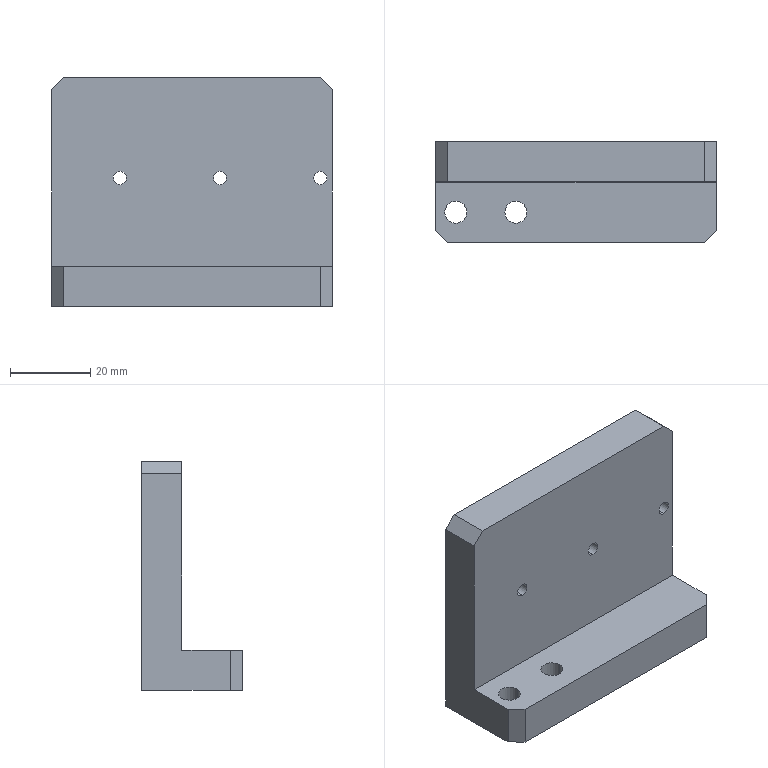Part | SolidWorks | features HoleWzd 2, Chamfer 1, Extrusion 1, ICE 1 | 1 solid | 22 faces | box 70 x 25 x 57 mm | volume 49488 mm3 | plane 12 | cylinder 10 | commonest cylinder face diameters 3.3 x6 5.5 x4
STEP:
#1=CARTESIAN_POINT('',(-17.75,-7.5,-28.5));
#2=VERTEX_POINT('',#1);
#3=CARTESIAN_POINT('',(-12.25,-7.5,-28.5));
#4=VERTEX_POINT('',#3);
#5=CARTESIAN_POINT('',(-15.,-7.5,-28.5));
#6=DIRECTION('',(0.,0.,1.));
#7=DIRECTION('',(1.,0.,0.));
#8=AXIS2_PLACEMENT_3D('',#5,#6,#7);
#9=CIRCLE('',#8,2.75);
#10=EDGE_CURVE('',#2,#4,#9,.T.);
#11=ORIENTED_EDGE('',*,*,#10,.F.);
#12=CARTESIAN_POINT('',(-17.75,-7.5,-18.5));
#13=VERTEX_POINT('',#12);
#14=CARTESIAN_POINT('',(-17.75,-7.5,-18.5));
#15=DIRECTION('',(0.,0.,1.));
#16=VECTOR('',#15,1000.);
#17=LINE('',#14,#16);
#18=EDGE_CURVE('',#2,#13,#17,.T.);
#19=ORIENTED_EDGE('',*,*,#18,.T.);
#20=CARTESIAN_POINT('',(-12.25,-7.5,-18.5));
#21=VERTEX_POINT('',#20);
#22=CARTESIAN_POINT('',(-15.,-7.5,-18.5));
#23=DIRECTION('',(0.,0.,1.));
#24=DIRECTION('',(1.,0.,0.));
#25=AXIS2_PLACEMENT_3D('',#22,#23,#24);
#26=CIRCLE('',#25,2.75);
#27=EDGE_CURVE('',#13,#21,#26,.T.);
#28=ORIENTED_EDGE('',*,*,#27,.T.);
#29=CARTESIAN_POINT('',(-12.25,-7.5,-18.5));
#30=DIRECTION('',(0.,0.,1.));
#31=VECTOR('',#30,1000.);
#32=LINE('',#29,#31);
#33=EDGE_CURVE('',#4,#21,#32,.T.);
#34=ORIENTED_EDGE('',*,*,#33,.F.);
#35=EDGE_LOOP('',(#11,#19,#28,#34));
#36=FACE_OUTER_BOUND('',#35,.T.);
#37=CARTESIAN_POINT('',(-15.,-7.5,-18.5));
#38=DIRECTION('',(0.,0.,1.));
#39=DIRECTION('',(1.,0.,0.));
#40=AXIS2_PLACEMENT_3D('',#37,#38,#39);
#41=CYLINDRICAL_SURFACE('',#40,2.75);
#42=ADVANCED_FACE('',(#36),#41,.F.);
#43=CARTESIAN_POINT('',(-32.75,-7.5,-28.5));
#44=VERTEX_POINT('',#43);
#45=CARTESIAN_POINT('',(-27.25,-7.5,-28.5));
#46=VERTEX_POINT('',#45);
#47=CARTESIAN_POINT('',(-30.,-7.5,-28.5));
#48=DIRECTION('',(0.,0.,1.));
#49=DIRECTION('',(1.,0.,0.));
#50=AXIS2_PLACEMENT_3D('',#47,#48,#49);
#51=CIRCLE('',#50,2.75);
#52=EDGE_CURVE('',#44,#46,#51,.T.);
#53=ORIENTED_EDGE('',*,*,#52,.F.);
#54=CARTESIAN_POINT('',(-32.75,-7.5,-18.5));
#55=VERTEX_POINT('',#54);
#56=CARTESIAN_POINT('',(-32.75,-7.5,-18.5));
#57=DIRECTION('',(0.,0.,1.));
#58=VECTOR('',#57,1000.);
#59=LINE('',#56,#58);
#60=EDGE_CURVE('',#44,#55,#59,.T.);
#61=ORIENTED_EDGE('',*,*,#60,.T.);
#62=CARTESIAN_POINT('',(-27.25,-7.5,-18.5));
#63=VERTEX_POINT('',#62);
#64=CARTESIAN_POINT('',(-30.,-7.5,-18.5));
#65=DIRECTION('',(0.,0.,1.));
#66=DIRECTION('',(1.,0.,0.));
#67=AXIS2_PLACEMENT_3D('',#64,#65,#66);
#68=CIRCLE('',#67,2.75);
#69=EDGE_CURVE('',#55,#63,#68,.T.);
#70=ORIENTED_EDGE('',*,*,#69,.T.);
#71=CARTESIAN_POINT('',(-27.25,-7.5,-18.5));
#72=DIRECTION('',(0.,0.,1.));
#73=VECTOR('',#72,1000.);
#74=LINE('',#71,#73);
#75=EDGE_CURVE('',#46,#63,#74,.T.);
#76=ORIENTED_EDGE('',*,*,#75,.F.);
#77=EDGE_LOOP('',(#53,#61,#70,#76));
#78=FACE_OUTER_BOUND('',#77,.T.);
#79=CARTESIAN_POINT('',(-30.,-7.5,-18.5));
#80=DIRECTION('',(0.,0.,1.));
#81=DIRECTION('',(1.,0.,0.));
#82=AXIS2_PLACEMENT_3D('',#79,#80,#81);
#83=CYLINDRICAL_SURFACE('',#82,2.75);
#84=ADVANCED_FACE('',(#78),#83,.F.);
#85=CARTESIAN_POINT('',(32.,0.,1.85));
#86=VERTEX_POINT('',#85);
#87=CARTESIAN_POINT('',(32.,0.,5.15));
#88=VERTEX_POINT('',#87);
#89=CARTESIAN_POINT('',(32.,0.,3.5));
#90=DIRECTION('',(0.,1.,0.));
#91=DIRECTION('',(0.,0.,1.));
#92=AXIS2_PLACEMENT_3D('',#89,#90,#91);
#93=CIRCLE('',#92,1.65);
#94=EDGE_CURVE('',#86,#88,#93,.T.);
#95=ORIENTED_EDGE('',*,*,#94,.F.);
#96=CARTESIAN_POINT('',(32.,10.,1.85));
#97=VERTEX_POINT('',#96);
#98=CARTESIAN_POINT('',(32.,10.,1.85));
#99=DIRECTION('',(0.,1.,0.));
#100=VECTOR('',#99,1000.);
#101=LINE('',#98,#100);
#102=EDGE_CURVE('',#86,#97,#101,.T.);
#103=ORIENTED_EDGE('',*,*,#102,.T.);
#104=CARTESIAN_POINT('',(32.,10.,5.15));
#105=VERTEX_POINT('',#104);
#106=CARTESIAN_POINT('',(32.,10.,3.5));
#107=DIRECTION('',(0.,1.,0.));
#108=DIRECTION('',(0.,0.,1.));
#109=AXIS2_PLACEMENT_3D('',#106,#107,#108);
#110=CIRCLE('',#109,1.65);
#111=EDGE_CURVE('',#97,#105,#110,.T.);
#112=ORIENTED_EDGE('',*,*,#111,.T.);
#113=CARTESIAN_POINT('',(32.,10.,5.15));
#114=DIRECTION('',(0.,1.,0.));
#115=VECTOR('',#114,1000.);
#116=LINE('',#113,#115);
#117=EDGE_CURVE('',#88,#105,#116,.T.);
#118=ORIENTED_EDGE('',*,*,#117,.F.);
#119=EDGE_LOOP('',(#95,#103,#112,#118));
#120=FACE_OUTER_BOUND('',#119,.T.);
#121=CARTESIAN_POINT('',(32.,10.,3.5));
#122=DIRECTION('',(0.,1.,0.));
#123=DIRECTION('',(0.,0.,1.));
#124=AXIS2_PLACEMENT_3D('',#121,#122,#123);
#125=CYLINDRICAL_SURFACE('',#124,1.65);
#126=ADVANCED_FACE('',(#120),#125,.F.);
#127=CARTESIAN_POINT('',(-18.,0.,1.85));
#128=VERTEX_POINT('',#127);
#129=CARTESIAN_POINT('',(-18.,0.,5.15));
#130=VERTEX_POINT('',#129);
#131=CARTESIAN_POINT('',(-18.,0.,3.5));
#132=DIRECTION('',(0.,1.,0.));
#133=DIRECTION('',(0.,0.,1.));
#134=AXIS2_PLACEMENT_3D('',#131,#132,#133);
#135=CIRCLE('',#134,1.65);
#136=EDGE_CURVE('',#128,#130,#135,.T.);
#137=ORIENTED_EDGE('',*,*,#136,.F.);
#138=CARTESIAN_POINT('',(-18.,10.,1.85));
#139=VERTEX_POINT('',#138);
#140=CARTESIAN_POINT('',(-18.,10.,1.85));
#141=DIRECTION('',(0.,1.,0.));
#142=VECTOR('',#141,1000.);
#143=LINE('',#140,#142);
#144=EDGE_CURVE('',#128,#139,#143,.T.);
#145=ORIENTED_EDGE('',*,*,#144,.T.);
#146=CARTESIAN_POINT('',(-18.,10.,5.15));
#147=VERTEX_POINT('',#146);
#148=CARTESIAN_POINT('',(-18.,10.,3.5));
#149=DIRECTION('',(0.,1.,0.));
#150=DIRECTION('',(0.,0.,1.));
#151=AXIS2_PLACEMENT_3D('',#148,#149,#150);
#152=CIRCLE('',#151,1.65);
#153=EDGE_CURVE('',#139,#147,#152,.T.);
#154=ORIENTED_EDGE('',*,*,#153,.T.);
#155=CARTESIAN_POINT('',(-18.,10.,5.15));
#156=DIRECTION('',(0.,1.,0.));
#157=VECTOR('',#156,1000.);
#158=LINE('',#155,#157);
#159=EDGE_CURVE('',#130,#147,#158,.T.);
#160=ORIENTED_EDGE('',*,*,#159,.F.);
#161=EDGE_LOOP('',(#137,#145,#154,#160));
#162=FACE_OUTER_BOUND('',#161,.T.);
#163=CARTESIAN_POINT('',(-18.,10.,3.5));
#164=DIRECTION('',(0.,1.,0.));
#165=DIRECTION('',(0.,0.,1.));
#166=AXIS2_PLACEMENT_3D('',#163,#164,#165);
#167=CYLINDRICAL_SURFACE('',#166,1.65);
#168=ADVANCED_FACE('',(#162),#167,.F.);
#169=CARTESIAN_POINT('',(7.,0.,1.85));
#170=VERTEX_POINT('',#169);
#171=CARTESIAN_POINT('',(7.,0.,5.15));
#172=VERTEX_POINT('',#171);
#173=CARTESIAN_POINT('',(7.,0.,3.5));
#174=DIRECTION('',(0.,1.,0.));
#175=DIRECTION('',(0.,0.,1.));
#176=AXIS2_PLACEMENT_3D('',#173,#174,#175);
#177=CIRCLE('',#176,1.65);
#178=EDGE_CURVE('',#170,#172,#177,.T.);
#179=ORIENTED_EDGE('',*,*,#178,.F.);
#180=CARTESIAN_POINT('',(7.,10.,1.85));
#181=VERTEX_POINT('',#180);
#182=CARTESIAN_POINT('',(7.,10.,1.85));
#183=DIRECTION('',(0.,1.,0.));
#184=VECTOR('',#183,1000.);
#185=LINE('',#182,#184);
#186=EDGE_CURVE('',#170,#181,#185,.T.);
#187=ORIENTED_EDGE('',*,*,#186,.T.);
#188=CARTESIAN_POINT('',(7.,10.,5.15));
#189=VERTEX_POINT('',#188);
#190=CARTESIAN_POINT('',(7.,10.,3.5));
#191=DIRECTION('',(0.,1.,0.));
#192=DIRECTION('',(0.,0.,1.));
#193=AXIS2_PLACEMENT_3D('',#190,#191,#192);
#194=CIRCLE('',#193,1.65);
#195=EDGE_CURVE('',#181,#189,#194,.T.);
#196=ORIENTED_EDGE('',*,*,#195,.T.);
#197=CARTESIAN_POINT('',(7.,10.,5.15));
#198=DIRECTION('',(0.,1.,0.));
#199=VECTOR('',#198,1000.);
#200=LINE('',#197,#199);
#201=EDGE_CURVE('',#172,#189,#200,.T.);
#202=ORIENTED_EDGE('',*,*,#201,.F.);
#203=EDGE_LOOP('',(#179,#187,#196,#202));
#204=FACE_OUTER_BOUND('',#203,.T.);
#205=CARTESIAN_POINT('',(7.,10.,3.5));
#206=DIRECTION('',(0.,1.,0.));
#207=DIRECTION('',(0.,0.,1.));
#208=AXIS2_PLACEMENT_3D('',#205,#206,#207);
#209=CYLINDRICAL_SURFACE('',#208,1.65);
#210=ADVANCED_FACE('',(#204),#209,.F.);
#211=CARTESIAN_POINT('',(32.,0.,3.5));
#212=DIRECTION('',(0.,1.,0.));
#213=DIRECTION('',(0.,0.,1.));
#214=AXIS2_PLACEMENT_3D('',#211,#212,#213);
#215=CIRCLE('',#214,1.65);
#216=EDGE_CURVE('',#88,#86,#215,.T.);
#217=ORIENTED_EDGE('',*,*,#216,.T.);
#218=ORIENTED_EDGE('',*,*,#94,.T.);
#219=EDGE_LOOP('',(#217,#218));
#220=FACE_BOUND('',#219,.T.);
#221=CARTESIAN_POINT('',(-18.,0.,3.5));
#222=DIRECTION('',(0.,1.,0.));
#223=DIRECTION('',(0.,0.,1.));
#224=AXIS2_PLACEMENT_3D('',#221,#222,#223);
#225=CIRCLE('',#224,1.65);
#226=EDGE_CURVE('',#130,#128,#225,.T.);
#227=ORIENTED_EDGE('',*,*,#226,.T.);
#228=ORIENTED_EDGE('',*,*,#136,.T.);
#229=EDGE_LOOP('',(#227,#228));
#230=FACE_BOUND('',#229,.T.);
#231=CARTESIAN_POINT('',(7.,0.,3.5));
#232=DIRECTION('',(0.,1.,0.));
#233=DIRECTION('',(0.,0.,1.));
#234=AXIS2_PLACEMENT_3D('',#231,#232,#233);
#235=CIRCLE('',#234,1.65);
#236=EDGE_CURVE('',#172,#170,#235,.T.);
#237=ORIENTED_EDGE('',*,*,#236,.T.);
#238=ORIENTED_EDGE('',*,*,#178,.T.);
#239=EDGE_LOOP('',(#237,#238));
#240=FACE_BOUND('',#239,.T.);
#241=CARTESIAN_POINT('',(-32.,0.,28.5));
#242=VERTEX_POINT('',#241);
#243=CARTESIAN_POINT('',(32.,0.,28.5));
#244=VERTEX_POINT('',#243);
#245=CARTESIAN_POINT('',(-35.,0.,28.5));
#246=DIRECTION('',(1.,0.,0.));
#247=VECTOR('',#246,1000.);
#248=LINE('',#245,#247);
#249=EDGE_CURVE('',#242,#244,#248,.T.);
#250=ORIENTED_EDGE('',*,*,#249,.F.);
#251=CARTESIAN_POINT('',(-35.,0.,25.5));
#252=VERTEX_POINT('',#251);
#253=CARTESIAN_POINT('',(-32.,0.,28.5));
#254=DIRECTION('',(-0.7071,0.,-0.7071));
#255=VECTOR('',#254,1000.);
#256=LINE('',#253,#255);
#257=EDGE_CURVE('',#242,#252,#256,.T.);
#258=ORIENTED_EDGE('',*,*,#257,.T.);
#259=CARTESIAN_POINT('',(-35.,0.,-18.5));
#260=VERTEX_POINT('',#259);
#261=CARTESIAN_POINT('',(-35.,0.,-28.5));
#262=DIRECTION('',(0.,0.,1.));
#263=VECTOR('',#262,1000.);
#264=LINE('',#261,#263);
#265=EDGE_CURVE('',#260,#252,#264,.T.);
#266=ORIENTED_EDGE('',*,*,#265,.F.);
#267=CARTESIAN_POINT('',(35.,0.,-18.5));
#268=VERTEX_POINT('',#267);
#269=CARTESIAN_POINT('',(35.,0.,-18.5));
#270=DIRECTION('',(-1.,0.,0.));
#271=VECTOR('',#270,1000.);
#272=LINE('',#269,#271);
#273=EDGE_CURVE('',#268,#260,#272,.T.);
#274=ORIENTED_EDGE('',*,*,#273,.F.);
#275=CARTESIAN_POINT('',(35.,0.,25.5));
#276=VERTEX_POINT('',#275);
#277=CARTESIAN_POINT('',(35.,0.,-28.5));
#278=DIRECTION('',(0.,0.,-1.));
#279=VECTOR('',#278,1000.);
#280=LINE('',#277,#279);
#281=EDGE_CURVE('',#276,#268,#280,.T.);
#282=ORIENTED_EDGE('',*,*,#281,.F.);
#283=CARTESIAN_POINT('',(35.,0.,25.5));
#284=DIRECTION('',(-0.7071,0.,0.7071));
#285=VECTOR('',#284,1000.);
#286=LINE('',#283,#285);
#287=EDGE_CURVE('',#276,#244,#286,.T.);
#288=ORIENTED_EDGE('',*,*,#287,.T.);
#289=EDGE_LOOP('',(#250,#258,#266,#274,#282,#288));
#290=FACE_OUTER_BOUND('',#289,.T.);
#291=CARTESIAN_POINT('',(0.,0.,0.));
#292=DIRECTION('',(0.,1.,0.));
#293=DIRECTION('',(0.,0.,1.));
#294=AXIS2_PLACEMENT_3D('',#291,#292,#293);
#295=PLANE('',#294);
#296=ADVANCED_FACE('',(#220,#230,#240,#290),#295,.F.);
#297=CARTESIAN_POINT('',(35.,10.,25.5));
#298=VERTEX_POINT('',#297);
#299=CARTESIAN_POINT('',(35.,10.,-28.5));
#300=VERTEX_POINT('',#299);
#301=CARTESIAN_POINT('',(35.,10.,-28.5));
#302=DIRECTION('',(0.,0.,-1.));
#303=VECTOR('',#302,1000.);
#304=LINE('',#301,#303);
#305=EDGE_CURVE('',#298,#300,#304,.T.);
#306=ORIENTED_EDGE('',*,*,#305,.F.);
#307=CARTESIAN_POINT('',(35.,10.,25.5));
#308=DIRECTION('',(0.,-1.,0.));
#309=VECTOR('',#308,1000.);
#310=LINE('',#307,#309);
#311=EDGE_CURVE('',#298,#276,#310,.T.);
#312=ORIENTED_EDGE('',*,*,#311,.T.);
#313=ORIENTED_EDGE('',*,*,#281,.T.);
#314=CARTESIAN_POINT('',(35.,-12.,-18.5));
#315=VERTEX_POINT('',#314);
#316=CARTESIAN_POINT('',(35.,-15.,-18.5));
#317=DIRECTION('',(0.,1.,0.));
#318=VECTOR('',#317,1000.);
#319=LINE('',#316,#318);
#320=EDGE_CURVE('',#315,#268,#319,.T.);
#321=ORIENTED_EDGE('',*,*,#320,.F.);
#322=CARTESIAN_POINT('',(35.,-12.,-28.5));
#323=VERTEX_POINT('',#322);
#324=CARTESIAN_POINT('',(35.,-12.,-28.5));
#325=DIRECTION('',(0.,0.,-1.));
#326=VECTOR('',#325,1000.);
#327=LINE('',#324,#326);
#328=EDGE_CURVE('',#315,#323,#327,.T.);
#329=ORIENTED_EDGE('',*,*,#328,.T.);
#330=CARTESIAN_POINT('',(35.,10.,-28.5));
#331=DIRECTION('',(0.,-1.,0.));
#332=VECTOR('',#331,1000.);
#333=LINE('',#330,#332);
#334=EDGE_CURVE('',#300,#323,#333,.T.);
#335=ORIENTED_EDGE('',*,*,#334,.F.);
#336=EDGE_LOOP('',(#306,#312,#313,#321,#329,#335));
#337=FACE_OUTER_BOUND('',#336,.T.);
#338=CARTESIAN_POINT('',(35.,10.,-28.5));
#339=DIRECTION('',(-1.,0.,0.));
#340=DIRECTION('',(0.,0.,1.));
#341=AXIS2_PLACEMENT_3D('',#338,#339,#340);
#342=PLANE('',#341);
#343=ADVANCED_FACE('',(#337),#342,.F.);
#344=CARTESIAN_POINT('',(-15.,-7.5,-28.5));
#345=DIRECTION('',(0.,0.,1.));
#346=DIRECTION('',(1.,0.,0.));
#347=AXIS2_PLACEMENT_3D('',#344,#345,#346);
#348=CIRCLE('',#347,2.75);
#349=EDGE_CURVE('',#4,#2,#348,.T.);
#350=ORIENTED_EDGE('',*,*,#349,.T.);
#351=ORIENTED_EDGE('',*,*,#10,.T.);
#352=EDGE_LOOP('',(#350,#351));
#353=FACE_BOUND('',#352,.T.);
#354=CARTESIAN_POINT('',(-30.,-7.5,-28.5));
#355=DIRECTION('',(0.,0.,1.));
#356=DIRECTION('',(1.,0.,0.));
#357=AXIS2_PLACEMENT_3D('',#354,#355,#356);
#358=CIRCLE('',#357,2.75);
#359=EDGE_CURVE('',#46,#44,#358,.T.);
#360=ORIENTED_EDGE('',*,*,#359,.T.);
#361=ORIENTED_EDGE('',*,*,#52,.T.);
#362=EDGE_LOOP('',(#360,#361));
#363=FACE_BOUND('',#362,.T.);
#364=CARTESIAN_POINT('',(-32.,-15.,-28.5));
#365=VERTEX_POINT('',#364);
#366=CARTESIAN_POINT('',(32.,-15.,-28.5));
#367=VERTEX_POINT('',#366);
#368=CARTESIAN_POINT('',(35.,-15.,-28.5));
#369=DIRECTION('',(1.,0.,0.));
#370=VECTOR('',#369,1000.);
#371=LINE('',#368,#370);
#372=EDGE_CURVE('',#365,#367,#371,.T.);
#373=ORIENTED_EDGE('',*,*,#372,.F.);
#374=CARTESIAN_POINT('',(-35.,-12.,-28.5));
#375=VERTEX_POINT('',#374);
#376=CARTESIAN_POINT('',(-32.,-15.,-28.5));
#377=DIRECTION('',(-0.7071,0.7071,0.));
#378=VECTOR('',#377,1000.);
#379=LINE('',#376,#378);
#380=EDGE_CURVE('',#365,#375,#379,.T.);
#381=ORIENTED_EDGE('',*,*,#380,.T.);
#382=CARTESIAN_POINT('',(-35.,10.,-28.5));
#383=VERTEX_POINT('',#382);
#384=CARTESIAN_POINT('',(-35.,10.,-28.5));
#385=DIRECTION('',(0.,-1.,0.));
#386=VECTOR('',#385,1000.);
#387=LINE('',#384,#386);
#388=EDGE_CURVE('',#383,#375,#387,.T.);
#389=ORIENTED_EDGE('',*,*,#388,.F.);
#390=CARTESIAN_POINT('',(-35.,10.,-28.5));
#391=DIRECTION('',(-1.,0.,0.));
#392=VECTOR('',#391,1000.);
#393=LINE('',#390,#392);
#394=EDGE_CURVE('',#300,#383,#393,.T.);
#395=ORIENTED_EDGE('',*,*,#394,.F.);
#396=ORIENTED_EDGE('',*,*,#334,.T.);
#397=CARTESIAN_POINT('',(32.,-15.,-28.5));
#398=DIRECTION('',(-0.7071,-0.7071,0.));
#399=VECTOR('',#398,1000.);
#400=LINE('',#397,#399);
#401=EDGE_CURVE('',#323,#367,#400,.T.);
#402=ORIENTED_EDGE('',*,*,#401,.T.);
#403=EDGE_LOOP('',(#373,#381,#389,#395,#396,#402));
#404=FACE_OUTER_BOUND('',#403,.T.);
#405=CARTESIAN_POINT('',(-35.,10.,-28.5));
#406=DIRECTION('',(0.,0.,1.));
#407=DIRECTION('',(1.,0.,0.));
#408=AXIS2_PLACEMENT_3D('',#405,#406,#407);
#409=PLANE('',#408);
#410=ADVANCED_FACE('',(#353,#363,#404),#409,.F.);
#411=ORIENTED_EDGE('',*,*,#388,.T.);
#412=CARTESIAN_POINT('',(-35.,-12.,-18.5));
#413=VERTEX_POINT('',#412);
#414=CARTESIAN_POINT('',(-35.,-12.,-18.5));
#415=DIRECTION('',(0.,0.,1.));
#416=VECTOR('',#415,1000.);
#417=LINE('',#414,#416);
#418=EDGE_CURVE('',#375,#413,#417,.T.);
#419=ORIENTED_EDGE('',*,*,#418,.T.);
#420=CARTESIAN_POINT('',(-35.,-15.,-18.5));
#421=DIRECTION('',(0.,1.,0.));
#422=VECTOR('',#421,1000.);
#423=LINE('',#420,#422);
#424=EDGE_CURVE('',#413,#260,#423,.T.);
#425=ORIENTED_EDGE('',*,*,#424,.T.);
#426=ORIENTED_EDGE('',*,*,#265,.T.);
#427=CARTESIAN_POINT('',(-35.,10.,25.5));
#428=VERTEX_POINT('',#427);
#429=CARTESIAN_POINT('',(-35.,10.,25.5));
#430=DIRECTION('',(0.,1.,0.));
#431=VECTOR('',#430,1000.);
#432=LINE('',#429,#431);
#433=EDGE_CURVE('',#252,#428,#432,.T.);
#434=ORIENTED_EDGE('',*,*,#433,.T.);
#435=CARTESIAN_POINT('',(-35.,10.,-28.5));
#436=DIRECTION('',(0.,0.,1.));
#437=VECTOR('',#436,1000.);
#438=LINE('',#435,#437);
#439=EDGE_CURVE('',#383,#428,#438,.T.);
#440=ORIENTED_EDGE('',*,*,#439,.F.);
#441=EDGE_LOOP('',(#411,#419,#425,#426,#434,#440));
#442=FACE_OUTER_BOUND('',#441,.T.);
#443=CARTESIAN_POINT('',(-35.,10.,-28.5));
#444=DIRECTION('',(1.,0.,0.));
#445=DIRECTION('',(0.,0.,-1.));
#446=AXIS2_PLACEMENT_3D('',#443,#444,#445);
#447=PLANE('',#446);
#448=ADVANCED_FACE('',(#442),#447,.F.);
#449=CARTESIAN_POINT('',(-32.,10.,28.5));
#450=VERTEX_POINT('',#449);
#451=CARTESIAN_POINT('',(32.,10.,28.5));
#452=VERTEX_POINT('',#451);
#453=CARTESIAN_POINT('',(-35.,10.,28.5));
#454=DIRECTION('',(1.,0.,0.));
#455=VECTOR('',#454,1000.);
#456=LINE('',#453,#455);
#457=EDGE_CURVE('',#450,#452,#456,.T.);
#458=ORIENTED_EDGE('',*,*,#457,.F.);
#459=CARTESIAN_POINT('',(-32.,10.,28.5));
#460=DIRECTION('',(0.,-1.,0.));
#461=VECTOR('',#460,1000.);
#462=LINE('',#459,#461);
#463=EDGE_CURVE('',#450,#242,#462,.T.);
#464=ORIENTED_EDGE('',*,*,#463,.T.);
#465=ORIENTED_EDGE('',*,*,#249,.T.);
#466=CARTESIAN_POINT('',(32.,10.,28.5));
#467=DIRECTION('',(0.,1.,0.));
#468=VECTOR('',#467,1000.);
#469=LINE('',#466,#468);
#470=EDGE_CURVE('',#244,#452,#469,.T.);
#471=ORIENTED_EDGE('',*,*,#470,.T.);
#472=EDGE_LOOP('',(#458,#464,#465,#471));
#473=FACE_OUTER_BOUND('',#472,.T.);
#474=CARTESIAN_POINT('',(-35.,10.,28.5));
#475=DIRECTION('',(0.,0.,-1.));
#476=DIRECTION('',(-1.,0.,0.));
#477=AXIS2_PLACEMENT_3D('',#474,#475,#476);
#478=PLANE('',#477);
#479=ADVANCED_FACE('',(#473),#478,.F.);
#480=CARTESIAN_POINT('',(32.,10.,3.5));
#481=DIRECTION('',(0.,1.,0.));
#482=DIRECTION('',(0.,0.,1.));
#483=AXIS2_PLACEMENT_3D('',#480,#481,#482);
#484=CIRCLE('',#483,1.65);
#485=EDGE_CURVE('',#105,#97,#484,.T.);
#486=ORIENTED_EDGE('',*,*,#485,.F.);
#487=ORIENTED_EDGE('',*,*,#111,.F.);
#488=EDGE_LOOP('',(#486,#487));
#489=FACE_BOUND('',#488,.T.);
#490=CARTESIAN_POINT('',(-18.,10.,3.5));
#491=DIRECTION('',(0.,1.,0.));
#492=DIRECTION('',(0.,0.,1.));
#493=AXIS2_PLACEMENT_3D('',#490,#491,#492);
#494=CIRCLE('',#493,1.65);
#495=EDGE_CURVE('',#147,#139,#494,.T.);
#496=ORIENTED_EDGE('',*,*,#495,.F.);
#497=ORIENTED_EDGE('',*,*,#153,.F.);
#498=EDGE_LOOP('',(#496,#497));
#499=FACE_BOUND('',#498,.T.);
#500=CARTESIAN_POINT('',(7.,10.,3.5));
#501=DIRECTION('',(0.,1.,0.));
#502=DIRECTION('',(0.,0.,1.));
#503=AXIS2_PLACEMENT_3D('',#500,#501,#502);
#504=CIRCLE('',#503,1.65);
#505=EDGE_CURVE('',#189,#181,#504,.T.);
#506=ORIENTED_EDGE('',*,*,#505,.F.);
#507=ORIENTED_EDGE('',*,*,#195,.F.);
#508=EDGE_LOOP('',(#506,#507));
#509=FACE_BOUND('',#508,.T.);
#510=ORIENTED_EDGE('',*,*,#439,.T.);
#511=CARTESIAN_POINT('',(-30.25,10.,30.25));
#512=DIRECTION('',(0.7071,0.,0.7071));
#513=VECTOR('',#512,1000.);
#514=LINE('',#511,#513);
#515=EDGE_CURVE('',#428,#450,#514,.T.);
#516=ORIENTED_EDGE('',*,*,#515,.T.);
#517=ORIENTED_EDGE('',*,*,#457,.T.);
#518=CARTESIAN_POINT('',(30.25,10.,30.25));
#519=DIRECTION('',(0.7071,0.,-0.7071));
#520=VECTOR('',#519,1000.);
#521=LINE('',#518,#520);
#522=EDGE_CURVE('',#452,#298,#521,.T.);
#523=ORIENTED_EDGE('',*,*,#522,.T.);
#524=ORIENTED_EDGE('',*,*,#305,.T.);
#525=ORIENTED_EDGE('',*,*,#394,.T.);
#526=EDGE_LOOP('',(#510,#516,#517,#523,#524,#525));
#527=FACE_OUTER_BOUND('',#526,.T.);
#528=CARTESIAN_POINT('',(0.,10.,0.));
#529=DIRECTION('',(0.,1.,0.));
#530=DIRECTION('',(0.,0.,1.));
#531=AXIS2_PLACEMENT_3D('',#528,#529,#530);
#532=PLANE('',#531);
#533=ADVANCED_FACE('',(#489,#499,#509,#527),#532,.T.);
#534=CARTESIAN_POINT('',(-15.,-7.5,-18.5));
#535=DIRECTION('',(0.,0.,1.));
#536=DIRECTION('',(1.,0.,0.));
#537=AXIS2_PLACEMENT_3D('',#534,#535,#536);
#538=CIRCLE('',#537,2.75);
#539=EDGE_CURVE('',#21,#13,#538,.T.);
#540=ORIENTED_EDGE('',*,*,#539,.F.);
#541=ORIENTED_EDGE('',*,*,#27,.F.);
#542=EDGE_LOOP('',(#540,#541));
#543=FACE_BOUND('',#542,.T.);
#544=CARTESIAN_POINT('',(-30.,-7.5,-18.5));
#545=DIRECTION('',(0.,0.,1.));
#546=DIRECTION('',(1.,0.,0.));
#547=AXIS2_PLACEMENT_3D('',#544,#545,#546);
#548=CIRCLE('',#547,2.75);
#549=EDGE_CURVE('',#63,#55,#548,.T.);
#550=ORIENTED_EDGE('',*,*,#549,.F.);
#551=ORIENTED_EDGE('',*,*,#69,.F.);
#552=EDGE_LOOP('',(#550,#551));
#553=FACE_BOUND('',#552,.T.);
#554=ORIENTED_EDGE('',*,*,#424,.F.);
#555=CARTESIAN_POINT('',(-32.,-15.,-18.5));
#556=VERTEX_POINT('',#555);
#557=CARTESIAN_POINT('',(-32.,-15.,-18.5));
#558=DIRECTION('',(0.7071,-0.7071,0.));
#559=VECTOR('',#558,1000.);
#560=LINE('',#557,#559);
#561=EDGE_CURVE('',#413,#556,#560,.T.);
#562=ORIENTED_EDGE('',*,*,#561,.T.);
#563=CARTESIAN_POINT('',(32.,-15.,-18.5));
#564=VERTEX_POINT('',#563);
#565=CARTESIAN_POINT('',(35.,-15.,-18.5));
#566=DIRECTION('',(-1.,0.,0.));
#567=VECTOR('',#566,1000.);
#568=LINE('',#565,#567);
#569=EDGE_CURVE('',#564,#556,#568,.T.);
#570=ORIENTED_EDGE('',*,*,#569,.F.);
#571=CARTESIAN_POINT('',(32.,-15.,-18.5));
#572=DIRECTION('',(0.7071,0.7071,0.));
#573=VECTOR('',#572,1000.);
#574=LINE('',#571,#573);
#575=EDGE_CURVE('',#564,#315,#574,.T.);
#576=ORIENTED_EDGE('',*,*,#575,.T.);
#577=ORIENTED_EDGE('',*,*,#320,.T.);
#578=ORIENTED_EDGE('',*,*,#273,.T.);
#579=EDGE_LOOP('',(#554,#562,#570,#576,#577,#578));
#580=FACE_OUTER_BOUND('',#579,.T.);
#581=CARTESIAN_POINT('',(35.,-15.,-18.5));
#582=DIRECTION('',(0.,0.,-1.));
#583=DIRECTION('',(-1.,0.,0.));
#584=AXIS2_PLACEMENT_3D('',#581,#582,#583);
#585=PLANE('',#584);
#586=ADVANCED_FACE('',(#543,#553,#580),#585,.F.);
#587=ORIENTED_EDGE('',*,*,#569,.T.);
#588=CARTESIAN_POINT('',(-32.,-15.,-28.5));
#589=DIRECTION('',(0.,0.,-1.));
#590=VECTOR('',#589,1000.);
#591=LINE('',#588,#590);
#592=EDGE_CURVE('',#556,#365,#591,.T.);
#593=ORIENTED_EDGE('',*,*,#592,.T.);
#594=ORIENTED_EDGE('',*,*,#372,.T.);
#595=CARTESIAN_POINT('',(32.,-15.,-18.5));
#596=DIRECTION('',(0.,0.,1.));
#597=VECTOR('',#596,1000.);
#598=LINE('',#595,#597);
#599=EDGE_CURVE('',#367,#564,#598,.T.);
#600=ORIENTED_EDGE('',*,*,#599,.T.);
#601=EDGE_LOOP('',(#587,#593,#594,#600));
#602=FACE_OUTER_BOUND('',#601,.T.);
#603=CARTESIAN_POINT('',(0.,-15.,0.));
#604=DIRECTION('',(0.,-1.,0.));
#605=DIRECTION('',(0.,0.,-1.));
#606=AXIS2_PLACEMENT_3D('',#603,#604,#605);
#607=PLANE('',#606);
#608=ADVANCED_FACE('',(#602),#607,.T.);
#609=ORIENTED_EDGE('',*,*,#561,.F.);
#610=ORIENTED_EDGE('',*,*,#418,.F.);
#611=ORIENTED_EDGE('',*,*,#380,.F.);
#612=ORIENTED_EDGE('',*,*,#592,.F.);
#613=EDGE_LOOP('',(#609,#610,#611,#612));
#614=FACE_OUTER_BOUND('',#613,.T.);
#615=CARTESIAN_POINT('',(-32.,-15.,0.));
#616=DIRECTION('',(-0.7071,-0.7071,0.));
#617=DIRECTION('',(0.,0.,1.));
#618=AXIS2_PLACEMENT_3D('',#615,#616,#617);
#619=PLANE('',#618);
#620=ADVANCED_FACE('',(#614),#619,.T.);
#621=ORIENTED_EDGE('',*,*,#515,.F.);
#622=ORIENTED_EDGE('',*,*,#433,.F.);
#623=ORIENTED_EDGE('',*,*,#257,.F.);
#624=ORIENTED_EDGE('',*,*,#463,.F.);
#625=EDGE_LOOP('',(#621,#622,#623,#624));
#626=FACE_OUTER_BOUND('',#625,.T.);
#627=CARTESIAN_POINT('',(-32.,10.,28.5));
#628=DIRECTION('',(0.7071,0.,-0.7071));
#629=DIRECTION('',(0.,-1.,0.));
#630=AXIS2_PLACEMENT_3D('',#627,#628,#629);
#631=PLANE('',#630);
#632=ADVANCED_FACE('',(#626),#631,.F.);
#633=ORIENTED_EDGE('',*,*,#522,.F.);
#634=ORIENTED_EDGE('',*,*,#470,.F.);
#635=ORIENTED_EDGE('',*,*,#287,.F.);
#636=ORIENTED_EDGE('',*,*,#311,.F.);
#637=EDGE_LOOP('',(#633,#634,#635,#636));
#638=FACE_OUTER_BOUND('',#637,.T.);
#639=CARTESIAN_POINT('',(35.,10.,25.5));
#640=DIRECTION('',(-0.7071,0.,-0.7071));
#641=DIRECTION('',(0.,-1.,0.));
#642=AXIS2_PLACEMENT_3D('',#639,#640,#641);
#643=PLANE('',#642);
#644=ADVANCED_FACE('',(#638),#643,.F.);
#645=ORIENTED_EDGE('',*,*,#401,.F.);
#646=ORIENTED_EDGE('',*,*,#328,.F.);
#647=ORIENTED_EDGE('',*,*,#575,.F.);
#648=ORIENTED_EDGE('',*,*,#599,.F.);
#649=EDGE_LOOP('',(#645,#646,#647,#648));
#650=FACE_OUTER_BOUND('',#649,.T.);
#651=CARTESIAN_POINT('',(32.,-15.,0.));
#652=DIRECTION('',(0.7071,-0.7071,0.));
#653=DIRECTION('',(0.,0.,-1.));
#654=AXIS2_PLACEMENT_3D('',#651,#652,#653);
#655=PLANE('',#654);
#656=ADVANCED_FACE('',(#650),#655,.T.);
#657=ORIENTED_EDGE('',*,*,#186,.F.);
#658=ORIENTED_EDGE('',*,*,#236,.F.);
#659=ORIENTED_EDGE('',*,*,#201,.T.);
#660=ORIENTED_EDGE('',*,*,#505,.T.);
#661=EDGE_LOOP('',(#657,#658,#659,#660));
#662=FACE_OUTER_BOUND('',#661,.T.);
#663=CARTESIAN_POINT('',(7.,10.,3.5));
#664=DIRECTION('',(0.,1.,0.));
#665=DIRECTION('',(0.,0.,1.));
#666=AXIS2_PLACEMENT_3D('',#663,#664,#665);
#667=CYLINDRICAL_SURFACE('',#666,1.65);
#668=ADVANCED_FACE('',(#662),#667,.F.);
#669=ORIENTED_EDGE('',*,*,#144,.F.);
#670=ORIENTED_EDGE('',*,*,#226,.F.);
#671=ORIENTED_EDGE('',*,*,#159,.T.);
#672=ORIENTED_EDGE('',*,*,#495,.T.);
#673=EDGE_LOOP('',(#669,#670,#671,#672));
#674=FACE_OUTER_BOUND('',#673,.T.);
#675=CARTESIAN_POINT('',(-18.,10.,3.5));
#676=DIRECTION('',(0.,1.,0.));
#677=DIRECTION('',(0.,0.,1.));
#678=AXIS2_PLACEMENT_3D('',#675,#676,#677);
#679=CYLINDRICAL_SURFACE('',#678,1.65);
#680=ADVANCED_FACE('',(#674),#679,.F.);
#681=ORIENTED_EDGE('',*,*,#102,.F.);
#682=ORIENTED_EDGE('',*,*,#216,.F.);
#683=ORIENTED_EDGE('',*,*,#117,.T.);
#684=ORIENTED_EDGE('',*,*,#485,.T.);
#685=EDGE_LOOP('',(#681,#682,#683,#684));
#686=FACE_OUTER_BOUND('',#685,.T.);
#687=CARTESIAN_POINT('',(32.,10.,3.5));
#688=DIRECTION('',(0.,1.,0.));
#689=DIRECTION('',(0.,0.,1.));
#690=AXIS2_PLACEMENT_3D('',#687,#688,#689);
#691=CYLINDRICAL_SURFACE('',#690,1.65);
#692=ADVANCED_FACE('',(#686),#691,.F.);
#693=ORIENTED_EDGE('',*,*,#60,.F.);
#694=ORIENTED_EDGE('',*,*,#359,.F.);
#695=ORIENTED_EDGE('',*,*,#75,.T.);
#696=ORIENTED_EDGE('',*,*,#549,.T.);
#697=EDGE_LOOP('',(#693,#694,#695,#696));
#698=FACE_OUTER_BOUND('',#697,.T.);
#699=CARTESIAN_POINT('',(-30.,-7.5,-18.5));
#700=DIRECTION('',(0.,0.,1.));
#701=DIRECTION('',(1.,0.,0.));
#702=AXIS2_PLACEMENT_3D('',#699,#700,#701);
#703=CYLINDRICAL_SURFACE('',#702,2.75);
#704=ADVANCED_FACE('',(#698),#703,.F.);
#705=ORIENTED_EDGE('',*,*,#18,.F.);
#706=ORIENTED_EDGE('',*,*,#349,.F.);
#707=ORIENTED_EDGE('',*,*,#33,.T.);
#708=ORIENTED_EDGE('',*,*,#539,.T.);
#709=EDGE_LOOP('',(#705,#706,#707,#708));
#710=FACE_OUTER_BOUND('',#709,.T.);
#711=CARTESIAN_POINT('',(-15.,-7.5,-18.5));
#712=DIRECTION('',(0.,0.,1.));
#713=DIRECTION('',(1.,0.,0.));
#714=AXIS2_PLACEMENT_3D('',#711,#712,#713);
#715=CYLINDRICAL_SURFACE('',#714,2.75);
#716=ADVANCED_FACE('',(#710),#715,.F.);
#717=CLOSED_SHELL('',(#42,#84,#126,#168,#210,#296,#343,#410,#448,#479,#533,#586,#608,#620,#632,#644,#656,#668,#680,#692,#704,#716));
#718=MANIFOLD_SOLID_BREP('',#717);
#719=CARTESIAN_POINT('',(0.,0.,0.));
#720=DIRECTION('',(0.,0.,1.));
#721=DIRECTION('',(1.,0.,0.));
#722=AXIS2_PLACEMENT_3D('',#719,#720,#721);
#723=(LENGTH_UNIT()NAMED_UNIT(*)SI_UNIT(.MILLI.,.METRE.));
#724=UNCERTAINTY_MEASURE_WITH_UNIT(LENGTH_MEASURE(0.00001),#723,'','');
#725=(NAMED_UNIT(*)PLANE_ANGLE_UNIT()SI_UNIT($,.RADIAN.));
#726=(NAMED_UNIT(*)SI_UNIT($,.STERADIAN.)SOLID_ANGLE_UNIT());
#727=(GEOMETRIC_REPRESENTATION_CONTEXT(3)GLOBAL_UNCERTAINTY_ASSIGNED_CONTEXT((#724))GLOBAL_UNIT_ASSIGNED_CONTEXT((#723,#725,#726))REPRESENTATION_CONTEXT('',''));
#728=ADVANCED_BREP_SHAPE_REPRESENTATION('',(#718,#722),#727);